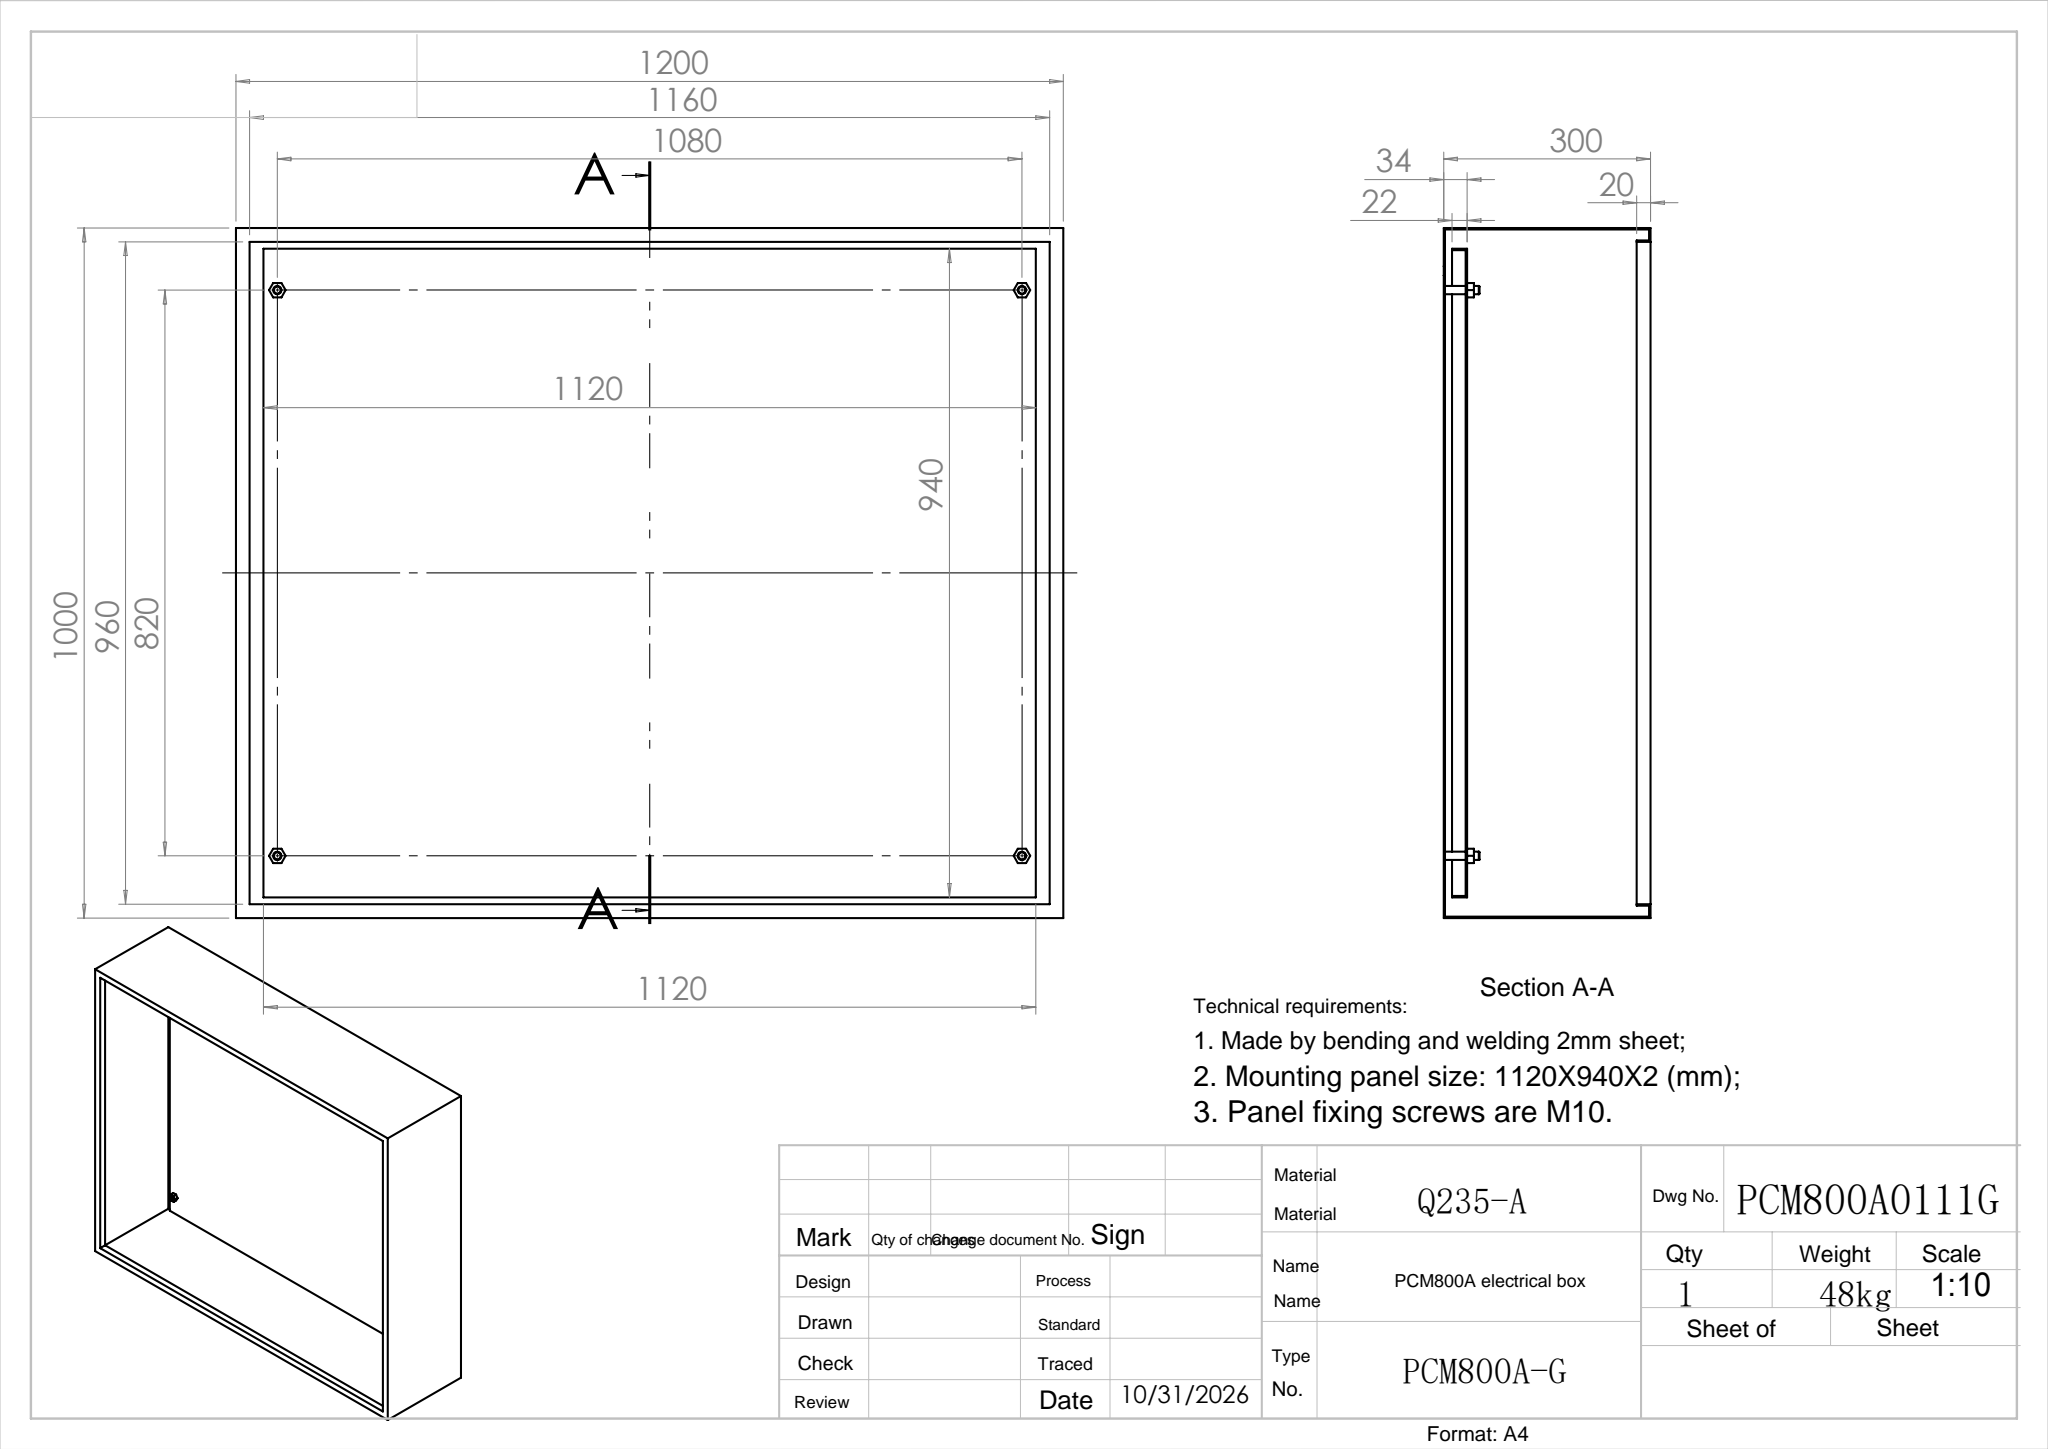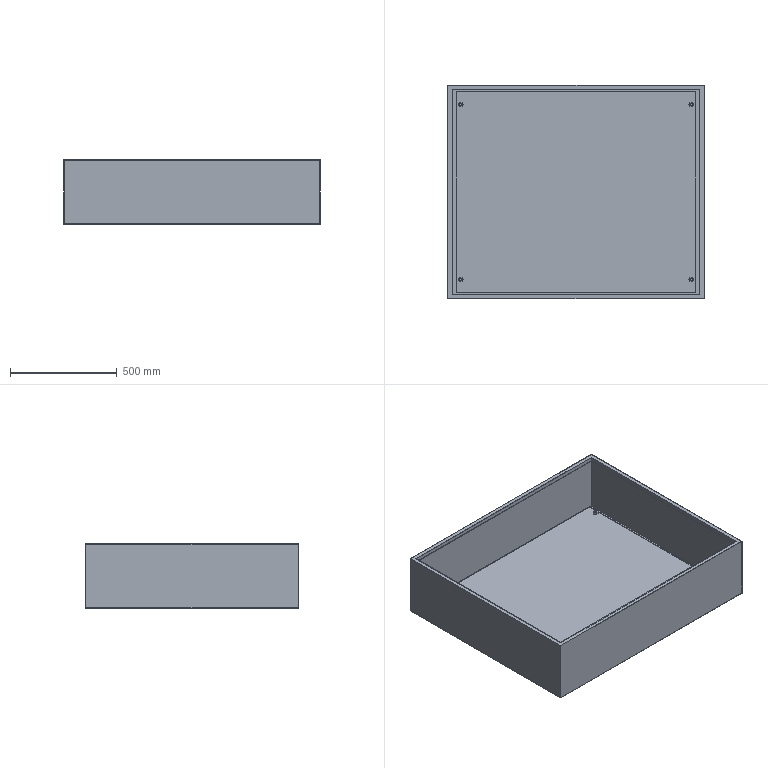Part | SolidWorks | features ICE 7, LPattern 3, Extrusion 1, Fillet 1, Shell 1 | 1 solid | 98 faces | box 1200 x 1000 x 300 mm | volume 7626457 mm3 | plane 64 | cylinder 26 | torus 8 | commonest cylinder face diameters 12 x16 14 x10